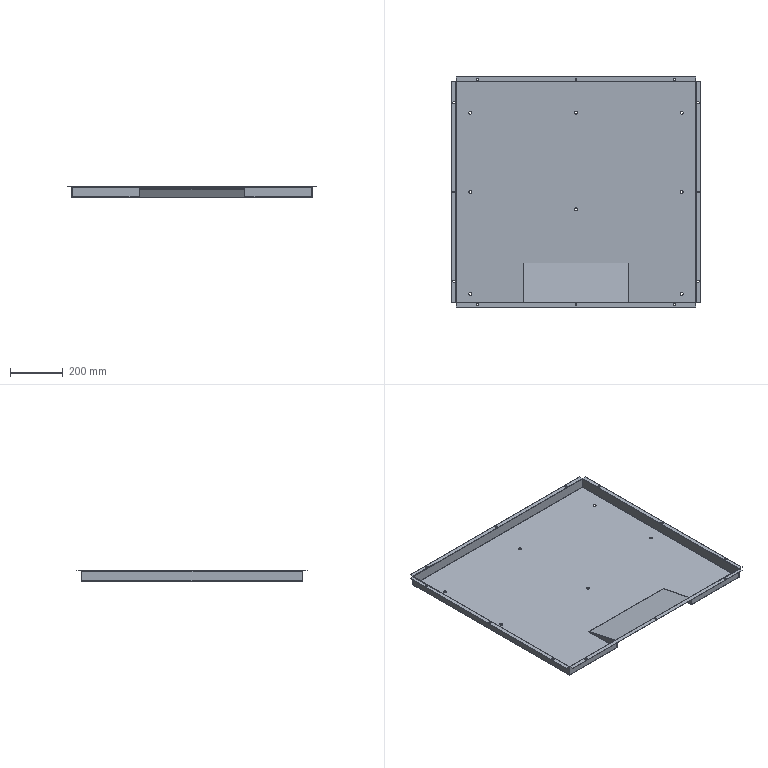Part | 2 solids | 170 faces | box 940 x 870 x 40 mm | volume 941829 mm3 | plane 90 | cylinder 68 | spline 12 | commonest cylinder face diameters 7 x30 11 x16 0.4 x9 2.4 x9 2 x2 4 x2